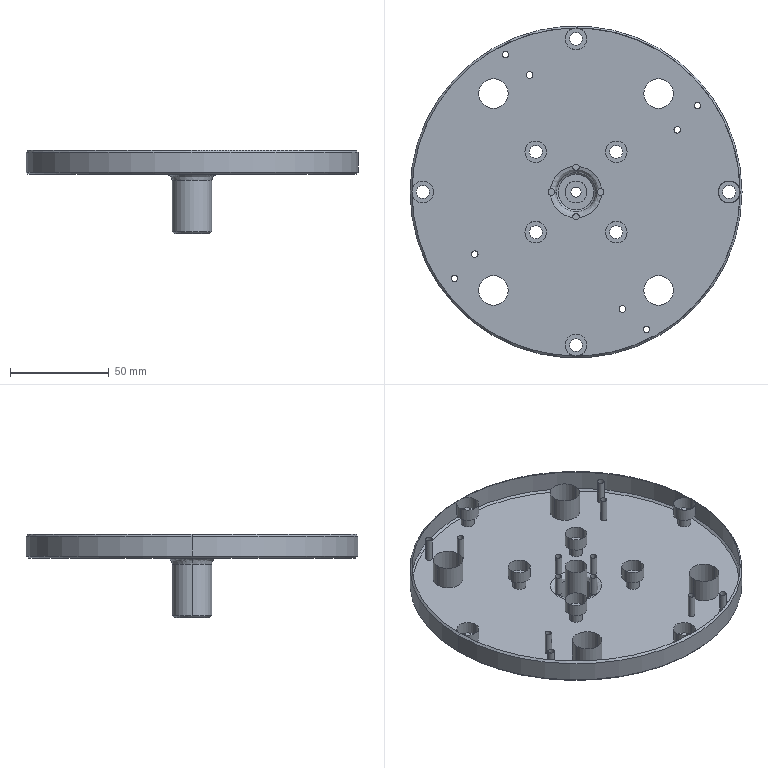Part | STEP file | Flange-10P30 | 1 solid | 96 faces | box 168 x 168 x 42 mm | volume 255273 mm3 | cylinder 72 | plane 16 | cone 6 | spline 2 | commonest cylinder face diameters 3.3 x24 6.6 x16 11 x16 15 x8 5.1 x2 11.1 x2